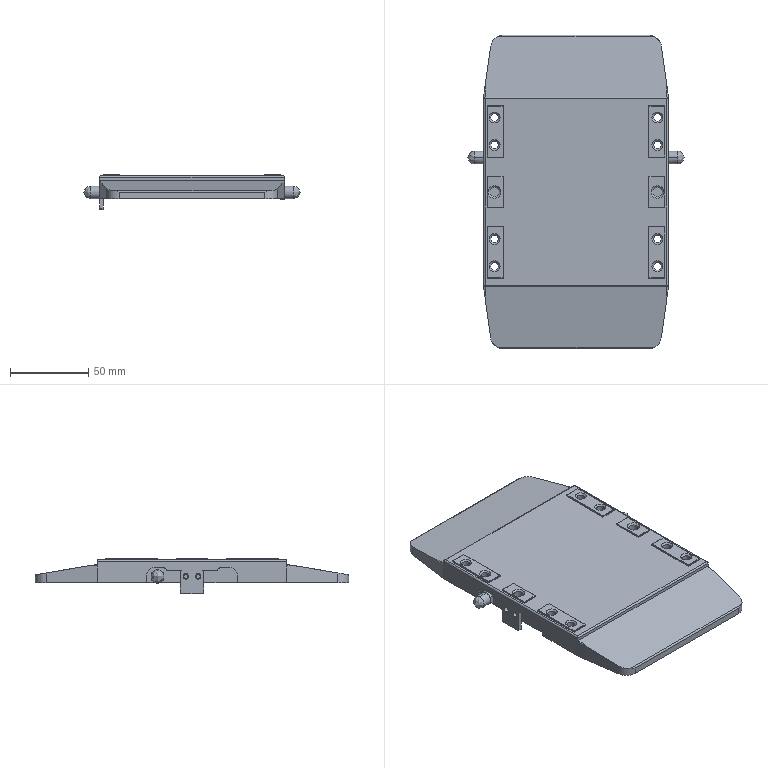Part | SolidWorks | features BaseBody 1 | 1 solid | 212 faces | box 137.84 x 200 x 22.5 mm | volume 281798 mm3 | plane 124 | cylinder 66 | cone 20 | spline 2 | commonest cylinder face diameters 2 x22 5 x16 2.5 x8 3.5 x4 6 x4 8 x4